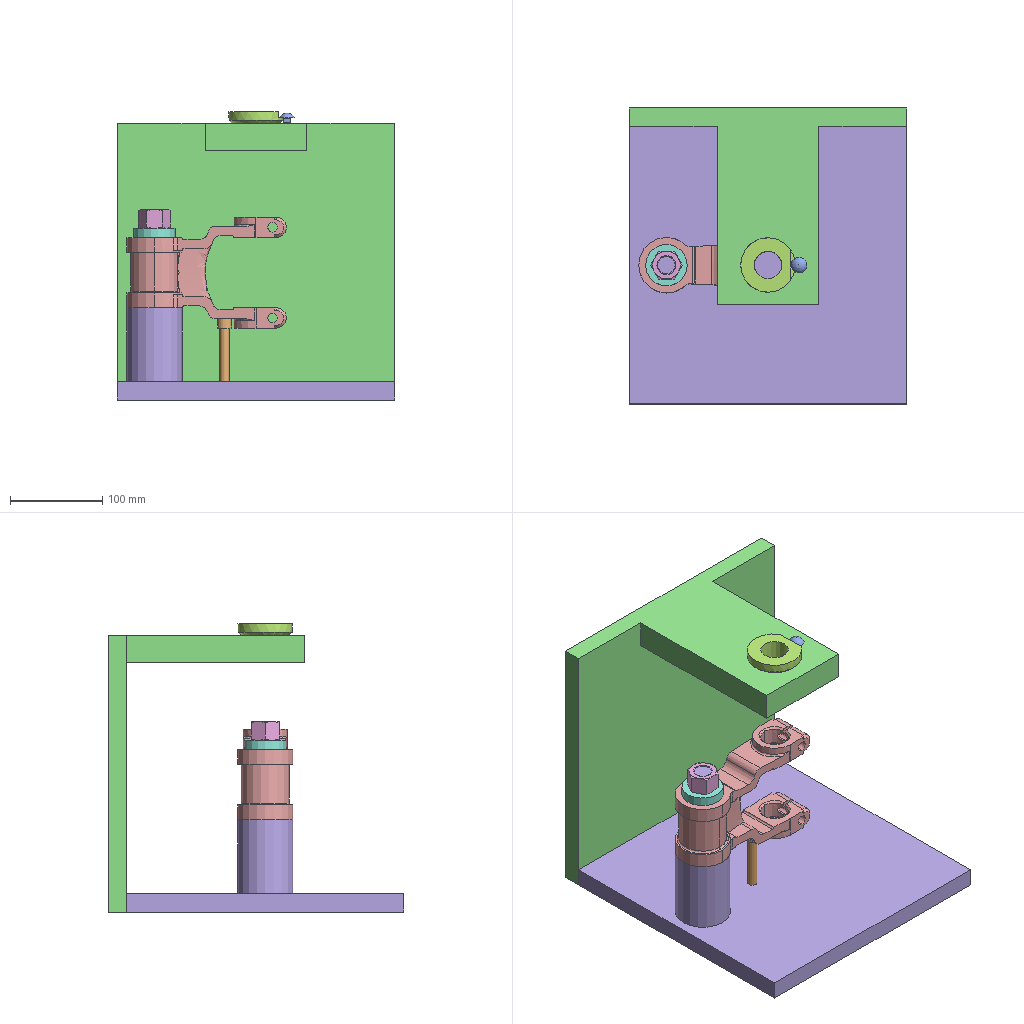Assembly | NX | 7 different items | 7 placed | box 300 x 320 x 312 mm
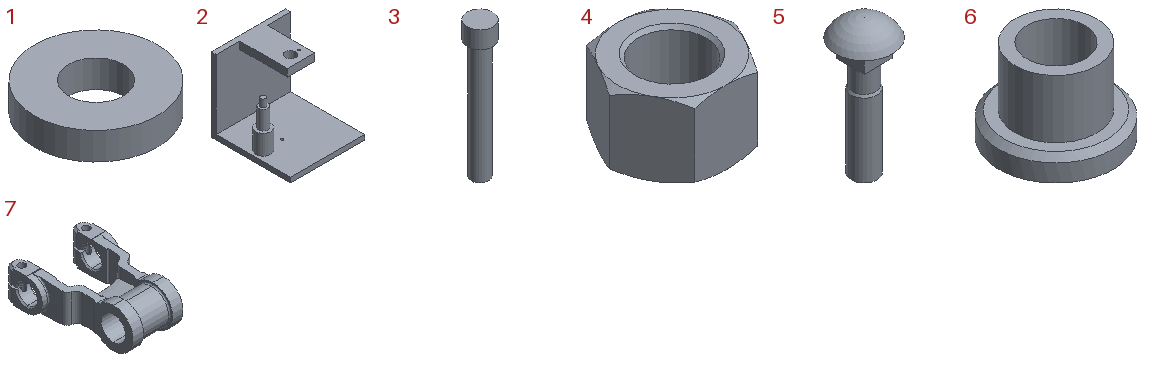Parts list (item | quantity | size | volume | features):
1 | x1 | 45 x 45 x 10 mm | 12763 mm3 | features DATUM_CSYS 2, EXTRUDE 1, SKETCH 1
2 | x1 | 300 x 320 x 300 mm | 4510024 mm3 | features DATUM_CSYS 16, SKETCH 15, EXTRUDE 6, SYMBOLIC_THREAD 2, HOLE PACKAGE 1, SIMPLE HOLE 1
3 | x1 | 15 x 15 x 79 mm | 7186 mm3 | features DATUM_CSYS 3, EXTRUDE 2, SKETCH 2, SYMBOLIC_THREAD 1
4 | x1 | 34.641 x 30 x 20.3 mm | 10084 mm3 | features META 3, SKETCH 3, DATUM_CSYS 2, EXTRUDE 2, SWP104 2, CHAMFER 1, LINE 1, SYMBOLIC_THREAD 1, THREADS 1
5 | x1 | 17.1 x 17.1 x 40.28 mm | 2398 mm3 | features DATUM_CSYS 2, SKETCH 2, BLEND 1, EXTRUDE 1, LINE 1, META 1, SWP104 1, SYMBOLIC_THREAD 1, THREADS 1
6 | x1 | 59 x 59 x 42 mm | 43152 mm3 | features DATUM_CSYS 4, EXTRUDE 3, SKETCH 3, CHAMFER 1
7 | x1 | 120 x 173 x 60 mm | 247159 mm3 | features DATUM_PLANE 8, DELETE FACE 6, DATUM_CSYS 4, SKETCH 3, TRIM BODY 3, CHAMFER 2, SPLIT BODY 2, UNITE 2, BLEND 1, BREP 1, Delete Body 1, EXTRUDE 1, MOVE_FACE 1, REPLACE_FACE 1, SKIN 1
Mates (type | each side: item.copy, entity, surface, feature):
Fix | 2.1 component
AlignLock | assembly face cylinder Extrude(2) | 2.1
Touch | assembly face plane Extrude(2) | 2.1
Touch | 3.1 face cylinder Extrude(2) | 2.1 face cylinder M10 x 1.5 Threaded Hole(18)
Touch | 1.1 face cylinder Extrude(2) | 2.1 face cylinder Extrude(14)
Touch | 1.1 face plane Extrude(2) | 2.1 face plane Extrude(12)
AlignLock | 4.1 face cylinder Extrude(8) | 2.1 face cylinder Extrude(14)
Touch | 4.1 face plane Extrude(5) | 1.1 face plane Extrude(2)
Parallel | 2.1 face plane Extrude(24) | 6.1 face plane Extrude(7)
AlignLock | 6.1 face cylinder Extrude(2) | 2.1 face cylinder Extrude(24)
Touch | 2.1 face plane Extrude(4) | 6.1 face plane Extrude(4)
AlignLock | 5.1 face cylinder Revolve(4) | 2.1 face cylinder Extrude(24)
Touch | 6.1 face plane Extrude(7) | 5.1 face plane Revolve(4)
AlignLock | 7.1 face cylinder Body(0) | 2.1 face cylinder Extrude(14)
Touch | 7.1 face plane Body(0) | 1.1 face plane Extrude(2)